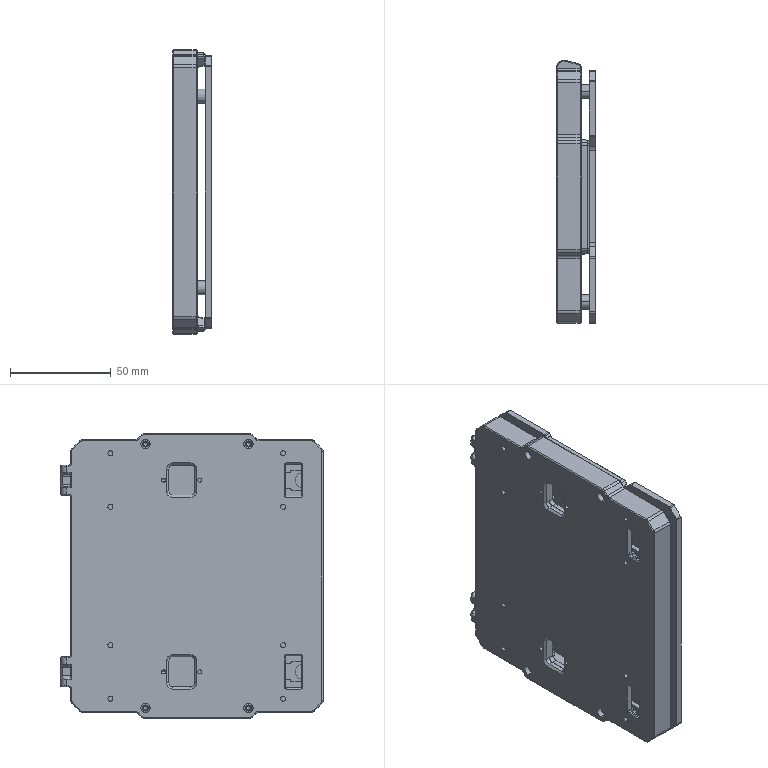Part | SolidWorks | features BaseBody 16, Blend 1, Shell 1 | 16 solids | 1245 faces | box 19 x 129.965 x 141 mm | volume 105960 mm3 | cylinder 564 | plane 465 | cone 112 | spline 88 | torus 16 | commonest cylinder face diameters 4 x152 1 x117 2 x74 3 x36 4.5 x24 6 x22